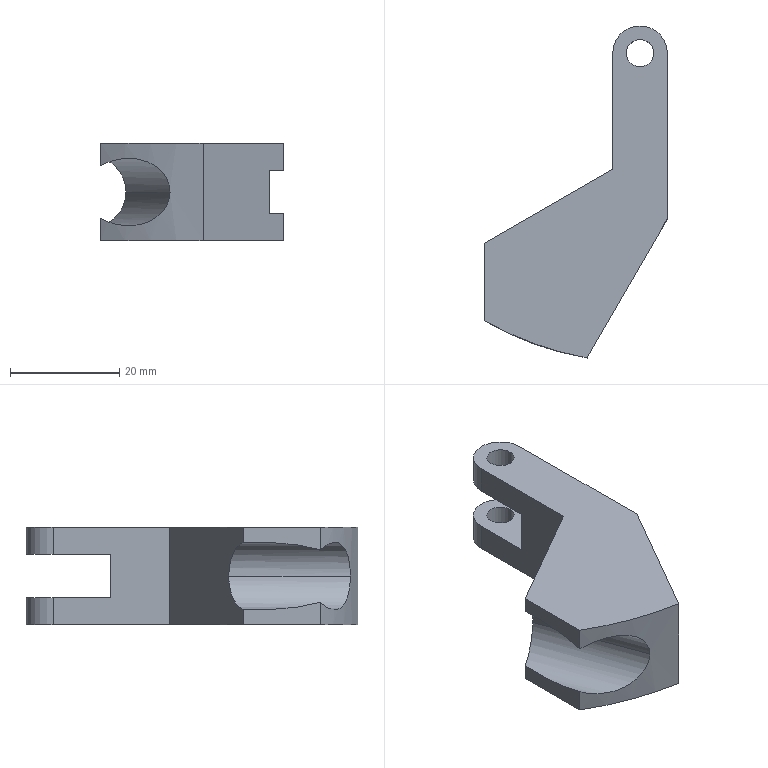Part | SolidWorks | features ICE 3, Extrusion 1 | 1 solid | 22 faces | box 33.5 x 60.913 x 17.9 mm | volume 14389 mm3 | plane 13 | cylinder 9 | commonest cylinder face diameters 5 x4 10 x2 12.4 x2 113.5 x1
STEP:
#1=CARTESIAN_POINT('',(-23.888,-32.221,8.95));
#2=VERTEX_POINT('',#1);
#3=CARTESIAN_POINT('',(-28.5,-34.884,15.076));
#4=VERTEX_POINT('',#3);
#5=CARTESIAN_POINT('',(-23.888,-32.221,8.95));
#6=CARTESIAN_POINT('',(-23.888,-32.221,12.151));
#7=CARTESIAN_POINT('',(-25.719,-33.278,14.583));
#8=CARTESIAN_POINT('',(-28.5,-34.884,15.076));
#9=(BOUNDED_CURVE()B_SPLINE_CURVE(3,(#5,#6,#7,#8),.UNSPECIFIED.,.F.,.F.)B_SPLINE_CURVE_WITH_KNOTS((4,4),(3.142,4.558),.UNSPECIFIED.)CURVE()GEOMETRIC_REPRESENTATION_ITEM()RATIONAL_B_SPLINE_CURVE((1.,0.8398,0.8398,1.))REPRESENTATION_ITEM(''));
#10=EDGE_CURVE('',#2,#4,#9,.T.);
#11=ORIENTED_EDGE('',*,*,#10,.F.);
#12=CARTESIAN_POINT('',(-15.774,-54.514,8.95));
#13=VERTEX_POINT('',#12);
#14=CARTESIAN_POINT('',(-26.37,-25.401,8.95));
#15=DIRECTION('',(0.342,-0.9397,0.));
#16=VECTOR('',#15,1000.);
#17=LINE('',#14,#16);
#18=EDGE_CURVE('',#2,#13,#17,.T.);
#19=ORIENTED_EDGE('',*,*,#18,.T.);
#20=CARTESIAN_POINT('',(-28.5,-49.075,13.771));
#21=VERTEX_POINT('',#20);
#22=CARTESIAN_POINT('',(-28.5,-49.075,13.771));
#23=CARTESIAN_POINT('',(-27.942,-49.399,14.106));
#24=CARTESIAN_POINT('',(-27.36,-49.724,14.372));
#25=CARTESIAN_POINT('',(-26.454,-50.208,14.688));
#26=CARTESIAN_POINT('',(-26.146,-50.369,14.778));
#27=CARTESIAN_POINT('',(-25.52,-50.689,14.932));
#28=CARTESIAN_POINT('',(-25.2,-50.849,14.994));
#29=CARTESIAN_POINT('',(-24.233,-51.321,15.136));
#30=CARTESIAN_POINT('',(-23.583,-51.623,15.17));
#31=CARTESIAN_POINT('',(-22.602,-52.056,15.124));
#32=CARTESIAN_POINT('',(-22.274,-52.197,15.092));
#33=CARTESIAN_POINT('',(-21.615,-52.473,14.994));
#34=CARTESIAN_POINT('',(-21.283,-52.609,14.926));
#35=CARTESIAN_POINT('',(-20.304,-52.998,14.667));
#36=CARTESIAN_POINT('',(-19.671,-53.236,14.422));
#37=CARTESIAN_POINT('',(-18.761,-53.56,13.92));
#38=CARTESIAN_POINT('',(-18.467,-53.662,13.73));
#39=CARTESIAN_POINT('',(-17.911,-53.85,13.31));
#40=CARTESIAN_POINT('',(-17.648,-53.937,13.079));
#41=CARTESIAN_POINT('',(-17.157,-54.095,12.571));
#42=CARTESIAN_POINT('',(-16.929,-54.166,12.292));
#43=CARTESIAN_POINT('',(-16.531,-54.289,11.702));
#44=CARTESIAN_POINT('',(-16.358,-54.342,11.39));
#45=CARTESIAN_POINT('',(-16.071,-54.427,10.725));
#46=CARTESIAN_POINT('',(-15.96,-54.459,10.38));
#47=CARTESIAN_POINT('',(-15.85,-54.492,9.853));
#48=CARTESIAN_POINT('',(-15.822,-54.5,9.675));
#49=CARTESIAN_POINT('',(-15.784,-54.511,9.315));
#50=CARTESIAN_POINT('',(-15.774,-54.514,9.132));
#51=CARTESIAN_POINT('',(-15.774,-54.514,8.95));
#52=B_SPLINE_CURVE_WITH_KNOTS('',3,(#22,#23,#24,#25,#26,#27,#28,#29,#30,#31,#32,#33,#34,#35,#36,#37,#38,#39,#40,#41,#42,#43,#44,#45,#46,#47,#48,#49,#50,#51),.UNSPECIFIED.,.F.,.F.,(4,2,2,2,2,2,2,2,2,2,2,2,2,2,4),(0.,0.002149,0.003224,0.004298,0.006447,0.007522,0.008597,0.01075,0.01182,0.01289,0.01397,0.01504,0.01612,0.01666,0.01719),.UNSPECIFIED.);
#53=EDGE_CURVE('',#21,#13,#52,.T.);
#54=ORIENTED_EDGE('',*,*,#53,.F.);
#55=CARTESIAN_POINT('',(-28.5,-34.884,15.076));
#56=CARTESIAN_POINT('',(-28.5,-40.017,15.35));
#57=CARTESIAN_POINT('',(-28.5,-45.034,14.889));
#58=CARTESIAN_POINT('',(-28.5,-49.075,13.771));
#59=(BOUNDED_CURVE()B_SPLINE_CURVE(3,(#55,#56,#57,#58),.UNSPECIFIED.,.F.,.F.)B_SPLINE_CURVE_WITH_KNOTS((4,4),(4.558,5.392),.UNSPECIFIED.)CURVE()GEOMETRIC_REPRESENTATION_ITEM()RATIONAL_B_SPLINE_CURVE((1.,0.9428,0.9428,1.))REPRESENTATION_ITEM(''));
#60=EDGE_CURVE('',#4,#21,#59,.T.);
#61=ORIENTED_EDGE('',*,*,#60,.F.);
#62=EDGE_LOOP('',(#11,#19,#54,#61));
#63=FACE_OUTER_BOUND('',#62,.T.);
#64=CARTESIAN_POINT('',(-32.196,-27.522,8.95));
#65=DIRECTION('',(0.342,-0.9397,0.));
#66=DIRECTION('',(0.9397,0.342,0.));
#67=AXIS2_PLACEMENT_3D('',#64,#65,#66);
#68=CYLINDRICAL_SURFACE('',#67,6.2);
#69=ADVANCED_FACE('',(#63),#68,.F.);
#70=CARTESIAN_POINT('',(-2.5,0.,17.9));
#71=VERTEX_POINT('',#70);
#72=CARTESIAN_POINT('',(2.5,0.,17.9));
#73=VERTEX_POINT('',#72);
#74=CARTESIAN_POINT('',(0.,0.,17.9));
#75=DIRECTION('',(0.,0.,1.));
#76=DIRECTION('',(1.,0.,0.));
#77=AXIS2_PLACEMENT_3D('',#74,#75,#76);
#78=CIRCLE('',#77,2.5);
#79=EDGE_CURVE('',#71,#73,#78,.T.);
#80=ORIENTED_EDGE('',*,*,#79,.T.);
#81=CARTESIAN_POINT('',(2.5,0.,12.9));
#82=VERTEX_POINT('',#81);
#83=CARTESIAN_POINT('',(2.5,0.,17.9));
#84=DIRECTION('',(0.,0.,-1.));
#85=VECTOR('',#84,1000.);
#86=LINE('',#83,#85);
#87=EDGE_CURVE('',#73,#82,#86,.T.);
#88=ORIENTED_EDGE('',*,*,#87,.T.);
#89=CARTESIAN_POINT('',(-2.5,0.,12.9));
#90=VERTEX_POINT('',#89);
#91=CARTESIAN_POINT('',(0.,0.,12.9));
#92=DIRECTION('',(0.,0.,1.));
#93=DIRECTION('',(1.,0.,0.));
#94=AXIS2_PLACEMENT_3D('',#91,#92,#93);
#95=CIRCLE('',#94,2.5);
#96=EDGE_CURVE('',#90,#82,#95,.T.);
#97=ORIENTED_EDGE('',*,*,#96,.F.);
#98=CARTESIAN_POINT('',(-2.5,0.,17.9));
#99=DIRECTION('',(0.,0.,-1.));
#100=VECTOR('',#99,1000.);
#101=LINE('',#98,#100);
#102=EDGE_CURVE('',#71,#90,#101,.T.);
#103=ORIENTED_EDGE('',*,*,#102,.F.);
#104=EDGE_LOOP('',(#80,#88,#97,#103));
#105=FACE_OUTER_BOUND('',#104,.T.);
#106=CARTESIAN_POINT('',(0.,0.,17.9));
#107=DIRECTION('',(0.,0.,-1.));
#108=DIRECTION('',(-1.,0.,0.));
#109=AXIS2_PLACEMENT_3D('',#106,#107,#108);
#110=CYLINDRICAL_SURFACE('',#109,2.5);
#111=ADVANCED_FACE('',(#105),#110,.F.);
#112=CARTESIAN_POINT('',(2.5,0.,5.));
#113=VERTEX_POINT('',#112);
#114=CARTESIAN_POINT('',(-2.5,0.,5.));
#115=VERTEX_POINT('',#114);
#116=CARTESIAN_POINT('',(0.,0.,5.));
#117=DIRECTION('',(0.,0.,-1.));
#118=DIRECTION('',(-1.,0.,0.));
#119=AXIS2_PLACEMENT_3D('',#116,#117,#118);
#120=CIRCLE('',#119,2.5);
#121=EDGE_CURVE('',#113,#115,#120,.T.);
#122=ORIENTED_EDGE('',*,*,#121,.F.);
#123=CARTESIAN_POINT('',(2.5,0.,0.));
#124=VERTEX_POINT('',#123);
#125=CARTESIAN_POINT('',(2.5,0.,17.9));
#126=DIRECTION('',(0.,0.,-1.));
#127=VECTOR('',#126,1000.);
#128=LINE('',#125,#127);
#129=EDGE_CURVE('',#113,#124,#128,.T.);
#130=ORIENTED_EDGE('',*,*,#129,.T.);
#131=CARTESIAN_POINT('',(-2.5,0.,0.));
#132=VERTEX_POINT('',#131);
#133=CARTESIAN_POINT('',(0.,0.,0.));
#134=DIRECTION('',(0.,0.,1.));
#135=DIRECTION('',(1.,0.,0.));
#136=AXIS2_PLACEMENT_3D('',#133,#134,#135);
#137=CIRCLE('',#136,2.5);
#138=EDGE_CURVE('',#132,#124,#137,.T.);
#139=ORIENTED_EDGE('',*,*,#138,.F.);
#140=CARTESIAN_POINT('',(-2.5,0.,17.9));
#141=DIRECTION('',(0.,0.,-1.));
#142=VECTOR('',#141,1000.);
#143=LINE('',#140,#142);
#144=EDGE_CURVE('',#115,#132,#143,.T.);
#145=ORIENTED_EDGE('',*,*,#144,.F.);
#146=EDGE_LOOP('',(#122,#130,#139,#145));
#147=FACE_OUTER_BOUND('',#146,.T.);
#148=CARTESIAN_POINT('',(0.,0.,17.9));
#149=DIRECTION('',(0.,0.,-1.));
#150=DIRECTION('',(-1.,0.,0.));
#151=AXIS2_PLACEMENT_3D('',#148,#149,#150);
#152=CYLINDRICAL_SURFACE('',#151,2.5);
#153=ADVANCED_FACE('',(#147),#152,.F.);
#154=CARTESIAN_POINT('',(-28.5,-49.075,4.129));
#155=VERTEX_POINT('',#154);
#156=CARTESIAN_POINT('',(-28.5,-49.075,0.));
#157=VERTEX_POINT('',#156);
#158=CARTESIAN_POINT('',(-28.5,-49.075,17.9));
#159=DIRECTION('',(0.,0.,-1.));
#160=VECTOR('',#159,1000.);
#161=LINE('',#158,#160);
#162=EDGE_CURVE('',#155,#157,#161,.T.);
#163=ORIENTED_EDGE('',*,*,#162,.F.);
#164=CARTESIAN_POINT('',(-28.5,-34.884,2.824));
#165=VERTEX_POINT('',#164);
#166=CARTESIAN_POINT('',(-28.5,-49.075,4.129));
#167=CARTESIAN_POINT('',(-28.5,-45.034,3.011));
#168=CARTESIAN_POINT('',(-28.5,-40.017,2.55));
#169=CARTESIAN_POINT('',(-28.5,-34.884,2.824));
#170=(BOUNDED_CURVE()B_SPLINE_CURVE(3,(#166,#167,#168,#169),.UNSPECIFIED.,.F.,.T.)B_SPLINE_CURVE_WITH_KNOTS((4,4),(0.8909,1.726),.UNSPECIFIED.)CURVE()GEOMETRIC_REPRESENTATION_ITEM()RATIONAL_B_SPLINE_CURVE((1.,0.9428,0.9428,1.))REPRESENTATION_ITEM(''));
#171=EDGE_CURVE('',#155,#165,#170,.T.);
#172=ORIENTED_EDGE('',*,*,#171,.T.);
#173=CARTESIAN_POINT('',(-28.5,-34.884,0.));
#174=VERTEX_POINT('',#173);
#175=CARTESIAN_POINT('',(-28.5,-34.884,17.9));
#176=DIRECTION('',(0.,0.,-1.));
#177=VECTOR('',#176,1000.);
#178=LINE('',#175,#177);
#179=EDGE_CURVE('',#165,#174,#178,.T.);
#180=ORIENTED_EDGE('',*,*,#179,.T.);
#181=CARTESIAN_POINT('',(-28.5,-34.884,0.));
#182=DIRECTION('',(0.,-1.,0.));
#183=VECTOR('',#182,1000.);
#184=LINE('',#181,#183);
#185=EDGE_CURVE('',#174,#157,#184,.T.);
#186=ORIENTED_EDGE('',*,*,#185,.T.);
#187=EDGE_LOOP('',(#163,#172,#180,#186));
#188=FACE_OUTER_BOUND('',#187,.T.);
#189=CARTESIAN_POINT('',(-28.5,-34.884,17.9));
#190=DIRECTION('',(1.,0.,0.));
#191=DIRECTION('',(0.,0.,-1.));
#192=AXIS2_PLACEMENT_3D('',#189,#190,#191);
#193=PLANE('',#192);
#194=ADVANCED_FACE('',(#188),#193,.F.);
#195=CARTESIAN_POINT('',(5.,0.,5.));
#196=VERTEX_POINT('',#195);
#197=CARTESIAN_POINT('',(5.,0.,0.));
#198=VERTEX_POINT('',#197);
#199=CARTESIAN_POINT('',(5.,0.,17.9));
#200=DIRECTION('',(0.,0.,-1.));
#201=VECTOR('',#200,1000.);
#202=LINE('',#199,#201);
#203=EDGE_CURVE('',#196,#198,#202,.T.);
#204=ORIENTED_EDGE('',*,*,#203,.F.);
#205=CARTESIAN_POINT('',(5.,-30.431,5.));
#206=VERTEX_POINT('',#205);
#207=CARTESIAN_POINT('',(5.,-30.431,5.));
#208=DIRECTION('',(0.,-1.,0.));
#209=VECTOR('',#208,1000.);
#210=LINE('',#207,#209);
#211=EDGE_CURVE('',#196,#206,#210,.T.);
#212=ORIENTED_EDGE('',*,*,#211,.T.);
#213=CARTESIAN_POINT('',(5.,-30.431,0.));
#214=VERTEX_POINT('',#213);
#215=CARTESIAN_POINT('',(5.,-30.431,17.9));
#216=DIRECTION('',(0.,0.,-1.));
#217=VECTOR('',#216,1000.);
#218=LINE('',#215,#217);
#219=EDGE_CURVE('',#206,#214,#218,.T.);
#220=ORIENTED_EDGE('',*,*,#219,.T.);
#221=CARTESIAN_POINT('',(5.,-30.431,0.));
#222=DIRECTION('',(0.,1.,0.));
#223=VECTOR('',#222,1000.);
#224=LINE('',#221,#223);
#225=EDGE_CURVE('',#214,#198,#224,.T.);
#226=ORIENTED_EDGE('',*,*,#225,.T.);
#227=EDGE_LOOP('',(#204,#212,#220,#226));
#228=FACE_OUTER_BOUND('',#227,.T.);
#229=CARTESIAN_POINT('',(5.,-30.431,17.9));
#230=DIRECTION('',(-1.,0.,0.));
#231=DIRECTION('',(0.,-1.,0.));
#232=AXIS2_PLACEMENT_3D('',#229,#230,#231);
#233=PLANE('',#232);
#234=ADVANCED_FACE('',(#228),#233,.F.);
#235=CARTESIAN_POINT('',(-5.,0.,5.));
#236=VERTEX_POINT('',#235);
#237=CARTESIAN_POINT('',(-5.,0.,0.));
#238=VERTEX_POINT('',#237);
#239=CARTESIAN_POINT('',(-5.,0.,17.9));
#240=DIRECTION('',(0.,0.,-1.));
#241=VECTOR('',#240,1000.);
#242=LINE('',#239,#241);
#243=EDGE_CURVE('',#236,#238,#242,.T.);
#244=ORIENTED_EDGE('',*,*,#243,.F.);
#245=CARTESIAN_POINT('',(0.,0.,5.));
#246=DIRECTION('',(0.,0.,-1.));
#247=DIRECTION('',(-1.,0.,0.));
#248=AXIS2_PLACEMENT_3D('',#245,#246,#247);
#249=CIRCLE('',#248,5.);
#250=EDGE_CURVE('',#236,#196,#249,.T.);
#251=ORIENTED_EDGE('',*,*,#250,.T.);
#252=ORIENTED_EDGE('',*,*,#203,.T.);
#253=CARTESIAN_POINT('',(0.,0.,0.));
#254=DIRECTION('',(0.,0.,1.));
#255=DIRECTION('',(1.,0.,0.));
#256=AXIS2_PLACEMENT_3D('',#253,#254,#255);
#257=CIRCLE('',#256,5.);
#258=EDGE_CURVE('',#198,#238,#257,.T.);
#259=ORIENTED_EDGE('',*,*,#258,.T.);
#260=EDGE_LOOP('',(#244,#251,#252,#259));
#261=FACE_OUTER_BOUND('',#260,.T.);
#262=CARTESIAN_POINT('',(0.,0.,17.9));
#263=DIRECTION('',(0.,0.,-1.));
#264=DIRECTION('',(-1.,0.,0.));
#265=AXIS2_PLACEMENT_3D('',#262,#263,#264);
#266=CYLINDRICAL_SURFACE('',#265,5.);
#267=ADVANCED_FACE('',(#261),#266,.T.);
#268=ORIENTED_EDGE('',*,*,#129,.F.);
#269=CARTESIAN_POINT('',(0.,0.,5.));
#270=DIRECTION('',(0.,0.,-1.));
#271=DIRECTION('',(-1.,0.,0.));
#272=AXIS2_PLACEMENT_3D('',#269,#270,#271);
#273=CIRCLE('',#272,2.5);
#274=EDGE_CURVE('',#115,#113,#273,.T.);
#275=ORIENTED_EDGE('',*,*,#274,.F.);
#276=ORIENTED_EDGE('',*,*,#144,.T.);
#277=CARTESIAN_POINT('',(0.,0.,0.));
#278=DIRECTION('',(0.,0.,1.));
#279=DIRECTION('',(1.,0.,0.));
#280=AXIS2_PLACEMENT_3D('',#277,#278,#279);
#281=CIRCLE('',#280,2.5);
#282=EDGE_CURVE('',#124,#132,#281,.T.);
#283=ORIENTED_EDGE('',*,*,#282,.F.);
#284=EDGE_LOOP('',(#268,#275,#276,#283));
#285=FACE_OUTER_BOUND('',#284,.T.);
#286=CARTESIAN_POINT('',(0.,0.,17.9));
#287=DIRECTION('',(0.,0.,-1.));
#288=DIRECTION('',(-1.,0.,0.));
#289=AXIS2_PLACEMENT_3D('',#286,#287,#288);
#290=CYLINDRICAL_SURFACE('',#289,2.5);
#291=ADVANCED_FACE('',(#285),#290,.F.);
#292=CARTESIAN_POINT('',(5.,-30.431,12.9));
#293=VERTEX_POINT('',#292);
#294=CARTESIAN_POINT('',(2.55,-34.675,12.9));
#295=VERTEX_POINT('',#294);
#296=CARTESIAN_POINT('',(2.55,-34.675,12.9));
#297=DIRECTION('',(-0.5,-0.866,0.));
#298=VECTOR('',#297,1000.);
#299=LINE('',#296,#298);
#300=EDGE_CURVE('',#293,#295,#299,.T.);
#301=ORIENTED_EDGE('',*,*,#300,.F.);
#302=CARTESIAN_POINT('',(5.,-30.431,17.9));
#303=VERTEX_POINT('',#302);
#304=CARTESIAN_POINT('',(5.,-30.431,17.9));
#305=DIRECTION('',(0.,0.,-1.));
#306=VECTOR('',#305,1000.);
#307=LINE('',#304,#306);
#308=EDGE_CURVE('',#303,#293,#307,.T.);
#309=ORIENTED_EDGE('',*,*,#308,.F.);
#310=CARTESIAN_POINT('',(-9.712,-55.913,17.9));
#311=VERTEX_POINT('',#310);
#312=CARTESIAN_POINT('',(-9.712,-55.913,17.9));
#313=DIRECTION('',(0.5,0.866,0.));
#314=VECTOR('',#313,1000.);
#315=LINE('',#312,#314);
#316=EDGE_CURVE('',#311,#303,#315,.T.);
#317=ORIENTED_EDGE('',*,*,#316,.F.);
#318=CARTESIAN_POINT('',(-9.712,-55.913,0.));
#319=VERTEX_POINT('',#318);
#320=CARTESIAN_POINT('',(-9.712,-55.913,17.9));
#321=DIRECTION('',(0.,0.,-1.));
#322=VECTOR('',#321,1000.);
#323=LINE('',#320,#322);
#324=EDGE_CURVE('',#311,#319,#323,.T.);
#325=ORIENTED_EDGE('',*,*,#324,.T.);
#326=CARTESIAN_POINT('',(-9.712,-55.913,0.));
#327=DIRECTION('',(0.5,0.866,0.));
#328=VECTOR('',#327,1000.);
#329=LINE('',#326,#328);
#330=EDGE_CURVE('',#319,#214,#329,.T.);
#331=ORIENTED_EDGE('',*,*,#330,.T.);
#332=ORIENTED_EDGE('',*,*,#219,.F.);
#333=CARTESIAN_POINT('',(2.55,-34.675,5.));
#334=VERTEX_POINT('',#333);
#335=CARTESIAN_POINT('',(2.55,-34.675,5.));
#336=DIRECTION('',(-0.5,-0.866,0.));
#337=VECTOR('',#336,1000.);
#338=LINE('',#335,#337);
#339=EDGE_CURVE('',#206,#334,#338,.T.);
#340=ORIENTED_EDGE('',*,*,#339,.T.);
#341=CARTESIAN_POINT('',(2.55,-34.675,12.9));
#342=DIRECTION('',(0.,0.,-1.));
#343=VECTOR('',#342,1000.);
#344=LINE('',#341,#343);
#345=EDGE_CURVE('',#295,#334,#344,.T.);
#346=ORIENTED_EDGE('',*,*,#345,.F.);
#347=EDGE_LOOP('',(#301,#309,#317,#325,#331,#332,#340,#346));
#348=FACE_OUTER_BOUND('',#347,.T.);
#349=CARTESIAN_POINT('',(-9.712,-55.913,17.9));
#350=DIRECTION('',(-0.866,0.5,0.));
#351=DIRECTION('',(-0.5,-0.866,0.));
#352=AXIS2_PLACEMENT_3D('',#349,#350,#351);
#353=PLANE('',#352);
#354=ADVANCED_FACE('',(#348),#353,.F.);
#355=CARTESIAN_POINT('',(5.,0.,12.9));
#356=VERTEX_POINT('',#355);
#357=CARTESIAN_POINT('',(5.,-30.431,12.9));
#358=DIRECTION('',(0.,-1.,0.));
#359=VECTOR('',#358,1000.);
#360=LINE('',#357,#359);
#361=EDGE_CURVE('',#356,#293,#360,.T.);
#362=ORIENTED_EDGE('',*,*,#361,.F.);
#363=CARTESIAN_POINT('',(5.,0.,17.9));
#364=VERTEX_POINT('',#363);
#365=CARTESIAN_POINT('',(5.,0.,17.9));
#366=DIRECTION('',(0.,0.,-1.));
#367=VECTOR('',#366,1000.);
#368=LINE('',#365,#367);
#369=EDGE_CURVE('',#364,#356,#368,.T.);
#370=ORIENTED_EDGE('',*,*,#369,.F.);
#371=CARTESIAN_POINT('',(5.,-30.431,17.9));
#372=DIRECTION('',(0.,1.,0.));
#373=VECTOR('',#372,1000.);
#374=LINE('',#371,#373);
#375=EDGE_CURVE('',#303,#364,#374,.T.);
#376=ORIENTED_EDGE('',*,*,#375,.F.);
#377=ORIENTED_EDGE('',*,*,#308,.T.);
#378=EDGE_LOOP('',(#362,#370,#376,#377));
#379=FACE_OUTER_BOUND('',#378,.T.);
#380=CARTESIAN_POINT('',(5.,-30.431,17.9));
#381=DIRECTION('',(-1.,0.,0.));
#382=DIRECTION('',(0.,-1.,0.));
#383=AXIS2_PLACEMENT_3D('',#380,#381,#382);
#384=PLANE('',#383);
#385=ADVANCED_FACE('',(#379),#384,.F.);
#386=CARTESIAN_POINT('',(-5.,0.,17.9));
#387=VERTEX_POINT('',#386);
#388=CARTESIAN_POINT('',(0.,0.,17.9));
#389=DIRECTION('',(0.,0.,1.));
#390=DIRECTION('',(1.,0.,0.));
#391=AXIS2_PLACEMENT_3D('',#388,#389,#390);
#392=CIRCLE('',#391,5.);
#393=EDGE_CURVE('',#364,#387,#392,.T.);
#394=ORIENTED_EDGE('',*,*,#393,.T.);
#395=CARTESIAN_POINT('',(-5.,-21.316,17.9));
#396=VERTEX_POINT('',#395);
#397=CARTESIAN_POINT('',(-5.,0.,17.9));
#398=DIRECTION('',(0.,-1.,0.));
#399=VECTOR('',#398,1000.);
#400=LINE('',#397,#399);
#401=EDGE_CURVE('',#387,#396,#400,.T.);
#402=ORIENTED_EDGE('',*,*,#401,.T.);
#403=CARTESIAN_POINT('',(-28.5,-34.884,17.9));
#404=VERTEX_POINT('',#403);
#405=CARTESIAN_POINT('',(-5.,-21.316,17.9));
#406=DIRECTION('',(-0.866,-0.5,0.));
#407=VECTOR('',#406,1000.);
#408=LINE('',#405,#407);
#409=EDGE_CURVE('',#396,#404,#408,.T.);
#410=ORIENTED_EDGE('',*,*,#409,.T.);
#411=CARTESIAN_POINT('',(-28.5,-49.075,17.9));
#412=VERTEX_POINT('',#411);
#413=CARTESIAN_POINT('',(-28.5,-34.884,17.9));
#414=DIRECTION('',(0.,-1.,0.));
#415=VECTOR('',#414,1000.);
#416=LINE('',#413,#415);
#417=EDGE_CURVE('',#404,#412,#416,.T.);
#418=ORIENTED_EDGE('',*,*,#417,.T.);
#419=CARTESIAN_POINT('',(0.,0.,17.9));
#420=DIRECTION('',(0.,0.,1.));
#421=DIRECTION('',(1.,0.,0.));
#422=AXIS2_PLACEMENT_3D('',#419,#420,#421);
#423=CIRCLE('',#422,56.75);
#424=EDGE_CURVE('',#412,#311,#423,.T.);
#425=ORIENTED_EDGE('',*,*,#424,.T.);
#426=ORIENTED_EDGE('',*,*,#316,.T.);
#427=ORIENTED_EDGE('',*,*,#375,.T.);
#428=EDGE_LOOP('',(#394,#402,#410,#418,#425,#426,#427));
#429=FACE_OUTER_BOUND('',#428,.T.);
#430=ORIENTED_EDGE('',*,*,#79,.F.);
#431=CARTESIAN_POINT('',(0.,0.,17.9));
#432=DIRECTION('',(0.,0.,1.));
#433=DIRECTION('',(1.,0.,0.));
#434=AXIS2_PLACEMENT_3D('',#431,#432,#433);
#435=CIRCLE('',#434,2.5);
#436=EDGE_CURVE('',#73,#71,#435,.T.);
#437=ORIENTED_EDGE('',*,*,#436,.F.);
#438=EDGE_LOOP('',(#430,#437));
#439=FACE_BOUND('',#438,.T.);
#440=CARTESIAN_POINT('',(0.,0.,17.9));
#441=DIRECTION('',(0.,0.,1.));
#442=DIRECTION('',(1.,0.,0.));
#443=AXIS2_PLACEMENT_3D('',#440,#441,#442);
#444=PLANE('',#443);
#445=ADVANCED_FACE('',(#429,#439),#444,.T.);
#446=ORIENTED_EDGE('',*,*,#258,.F.);
#447=ORIENTED_EDGE('',*,*,#225,.F.);
#448=ORIENTED_EDGE('',*,*,#330,.F.);
#449=CARTESIAN_POINT('',(0.,0.,0.));
#450=DIRECTION('',(0.,0.,1.));
#451=DIRECTION('',(1.,0.,0.));
#452=AXIS2_PLACEMENT_3D('',#449,#450,#451);
#453=CIRCLE('',#452,56.75);
#454=EDGE_CURVE('',#157,#319,#453,.T.);
#455=ORIENTED_EDGE('',*,*,#454,.F.);
#456=ORIENTED_EDGE('',*,*,#185,.F.);
#457=CARTESIAN_POINT('',(-5.,-21.316,0.));
#458=VERTEX_POINT('',#457);
#459=CARTESIAN_POINT('',(-5.,-21.316,0.));
#460=DIRECTION('',(-0.866,-0.5,0.));
#461=VECTOR('',#460,1000.);
#462=LINE('',#459,#461);
#463=EDGE_CURVE('',#458,#174,#462,.T.);
#464=ORIENTED_EDGE('',*,*,#463,.F.);
#465=CARTESIAN_POINT('',(-5.,0.,0.));
#466=DIRECTION('',(0.,-1.,0.));
#467=VECTOR('',#466,1000.);
#468=LINE('',#465,#467);
#469=EDGE_CURVE('',#238,#458,#468,.T.);
#470=ORIENTED_EDGE('',*,*,#469,.F.);
#471=EDGE_LOOP('',(#446,#447,#448,#455,#456,#464,#470));
#472=FACE_OUTER_BOUND('',#471,.T.);
#473=ORIENTED_EDGE('',*,*,#138,.T.);
#474=ORIENTED_EDGE('',*,*,#282,.T.);
#475=EDGE_LOOP('',(#473,#474));
#476=FACE_BOUND('',#475,.T.);
#477=CARTESIAN_POINT('',(0.,0.,0.));
#478=DIRECTION('',(0.,0.,1.));
#479=DIRECTION('',(1.,0.,0.));
#480=AXIS2_PLACEMENT_3D('',#477,#478,#479);
#481=PLANE('',#480);
#482=ADVANCED_FACE('',(#472,#476),#481,.F.);
#483=ORIENTED_EDGE('',*,*,#369,.T.);
#484=CARTESIAN_POINT('',(-5.,0.,12.9));
#485=VERTEX_POINT('',#484);
#486=CARTESIAN_POINT('',(0.,0.,12.9));
#487=DIRECTION('',(0.,0.,1.));
#488=DIRECTION('',(1.,0.,0.));
#489=AXIS2_PLACEMENT_3D('',#486,#487,#488);
#490=CIRCLE('',#489,5.);
#491=EDGE_CURVE('',#356,#485,#490,.T.);
#492=ORIENTED_EDGE('',*,*,#491,.T.);
#493=CARTESIAN_POINT('',(-5.,0.,17.9));
#494=DIRECTION('',(0.,0.,-1.));
#495=VECTOR('',#494,1000.);
#496=LINE('',#493,#495);
#497=EDGE_CURVE('',#387,#485,#496,.T.);
#498=ORIENTED_EDGE('',*,*,#497,.F.);
#499=ORIENTED_EDGE('',*,*,#393,.F.);
#500=EDGE_LOOP('',(#483,#492,#498,#499));
#501=FACE_OUTER_BOUND('',#500,.T.);
#502=CARTESIAN_POINT('',(0.,0.,17.9));
#503=DIRECTION('',(0.,0.,-1.));
#504=DIRECTION('',(-1.,0.,0.));
#505=AXIS2_PLACEMENT_3D('',#502,#503,#504);
#506=CYLINDRICAL_SURFACE('',#505,5.);
#507=ADVANCED_FACE('',(#501),#506,.T.);
#508=CARTESIAN_POINT('',(-5.,-10.556,5.));
#509=VERTEX_POINT('',#508);
#510=CARTESIAN_POINT('',(-5.,-10.556,12.9));
#511=VERTEX_POINT('',#510);
#512=CARTESIAN_POINT('',(-5.,-10.556,5.));
#513=DIRECTION('',(0.,0.,1.));
#514=VECTOR('',#513,1000.);
#515=LINE('',#512,#514);
#516=EDGE_CURVE('',#509,#511,#515,.T.);
#517=ORIENTED_EDGE('',*,*,#516,.F.);
#518=CARTESIAN_POINT('',(-5.,-10.556,5.));
#519=DIRECTION('',(0.,-1.,0.));
#520=VECTOR('',#519,1000.);
#521=LINE('',#518,#520);
#522=EDGE_CURVE('',#236,#509,#521,.T.);
#523=ORIENTED_EDGE('',*,*,#522,.F.);
#524=ORIENTED_EDGE('',*,*,#243,.T.);
#525=ORIENTED_EDGE('',*,*,#469,.T.);
#526=CARTESIAN_POINT('',(-5.,-21.316,17.9));
#527=DIRECTION('',(0.,0.,-1.));
#528=VECTOR('',#527,1000.);
#529=LINE('',#526,#528);
#530=EDGE_CURVE('',#396,#458,#529,.T.);
#531=ORIENTED_EDGE('',*,*,#530,.F.);
#532=ORIENTED_EDGE('',*,*,#401,.F.);
#533=ORIENTED_EDGE('',*,*,#497,.T.);
#534=CARTESIAN_POINT('',(-5.,7.33,12.9));
#535=DIRECTION('',(0.,1.,0.));
#536=VECTOR('',#535,1000.);
#537=LINE('',#534,#536);
#538=EDGE_CURVE('',#511,#485,#537,.T.);
#539=ORIENTED_EDGE('',*,*,#538,.F.);
#540=EDGE_LOOP('',(#517,#523,#524,#525,#531,#532,#533,#539));
#541=FACE_OUTER_BOUND('',#540,.T.);
#542=CARTESIAN_POINT('',(-5.,0.,17.9));
#543=DIRECTION('',(1.,0.,0.));
#544=DIRECTION('',(0.,1.,0.));
#545=AXIS2_PLACEMENT_3D('',#542,#543,#544);
#546=PLANE('',#545);
#547=ADVANCED_FACE('',(#541),#546,.F.);
#548=ORIENTED_EDGE('',*,*,#179,.F.);
#549=CARTESIAN_POINT('',(-28.5,-34.884,2.824));
#550=CARTESIAN_POINT('',(-25.719,-33.278,3.317));
#551=CARTESIAN_POINT('',(-23.888,-32.221,5.749));
#552=CARTESIAN_POINT('',(-23.888,-32.221,8.95));
#553=(BOUNDED_CURVE()B_SPLINE_CURVE(3,(#549,#550,#551,#552),.UNSPECIFIED.,.F.,.F.)B_SPLINE_CURVE_WITH_KNOTS((4,4),(1.726,3.142),.UNSPECIFIED.)CURVE()GEOMETRIC_REPRESENTATION_ITEM()RATIONAL_B_SPLINE_CURVE((1.,0.8398,0.8398,1.))REPRESENTATION_ITEM(''));
#554=EDGE_CURVE('',#165,#2,#553,.T.);
#555=ORIENTED_EDGE('',*,*,#554,.T.);
#556=ORIENTED_EDGE('',*,*,#10,.T.);
#557=CARTESIAN_POINT('',(-28.5,-34.884,17.9));
#558=DIRECTION('',(0.,0.,-1.));
#559=VECTOR('',#558,1000.);
#560=LINE('',#557,#559);
#561=EDGE_CURVE('',#404,#4,#560,.T.);
#562=ORIENTED_EDGE('',*,*,#561,.F.);
#563=ORIENTED_EDGE('',*,*,#409,.F.);
#564=ORIENTED_EDGE('',*,*,#530,.T.);
#565=ORIENTED_EDGE('',*,*,#463,.T.);
#566=EDGE_LOOP('',(#548,#555,#556,#562,#563,#564,#565));
#567=FACE_OUTER_BOUND('',#566,.T.);
#568=CARTESIAN_POINT('',(-5.,-21.316,17.9));
#569=DIRECTION('',(0.5,-0.866,0.));
#570=DIRECTION('',(0.866,0.5,0.));
#571=AXIS2_PLACEMENT_3D('',#568,#569,#570);
#572=PLANE('',#571);
#573=ADVANCED_FACE('',(#567),#572,.F.);
#574=ORIENTED_EDGE('',*,*,#561,.T.);
#575=ORIENTED_EDGE('',*,*,#60,.T.);
#576=CARTESIAN_POINT('',(-28.5,-49.075,17.9));
#577=DIRECTION('',(0.,0.,-1.));
#578=VECTOR('',#577,1000.);
#579=LINE('',#576,#578);
#580=EDGE_CURVE('',#412,#21,#579,.T.);
#581=ORIENTED_EDGE('',*,*,#580,.F.);
#582=ORIENTED_EDGE('',*,*,#417,.F.);
#583=EDGE_LOOP('',(#574,#575,#581,#582));
#584=FACE_OUTER_BOUND('',#583,.T.);
#585=CARTESIAN_POINT('',(-28.5,-34.884,17.9));
#586=DIRECTION('',(1.,0.,0.));
#587=DIRECTION('',(0.,0.,-1.));
#588=AXIS2_PLACEMENT_3D('',#585,#586,#587);
#589=PLANE('',#588);
#590=ADVANCED_FACE('',(#584),#589,.F.);
#591=ORIENTED_EDGE('',*,*,#580,.T.);
#592=ORIENTED_EDGE('',*,*,#53,.T.);
#593=CARTESIAN_POINT('',(-15.774,-54.514,8.95));
#594=CARTESIAN_POINT('',(-15.774,-54.514,8.586));
#595=CARTESIAN_POINT('',(-15.812,-54.503,8.228));
#596=CARTESIAN_POINT('',(-15.96,-54.46,7.523));
#597=CARTESIAN_POINT('',(-16.071,-54.427,7.174));
#598=CARTESIAN_POINT('',(-16.355,-54.342,6.516));
#599=CARTESIAN_POINT('',(-16.527,-54.29,6.203));
#600=CARTESIAN_POINT('',(-16.929,-54.166,5.608));
#601=CARTESIAN_POINT('',(-17.154,-54.096,5.333));
#602=CARTESIAN_POINT('',(-17.643,-53.938,4.826));
#603=CARTESIAN_POINT('',(-17.909,-53.851,4.591));
#604=CARTESIAN_POINT('',(-18.467,-53.662,4.17));
#605=CARTESIAN_POINT('',(-18.758,-53.561,3.983));
#606=CARTESIAN_POINT('',(-19.357,-53.348,3.651));
#607=CARTESIAN_POINT('',(-19.666,-53.235,3.506));
#608=CARTESIAN_POINT('',(-20.302,-52.995,3.254));
#609=CARTESIAN_POINT('',(-20.626,-52.87,3.148));
#610=CARTESIAN_POINT('',(-21.599,-52.484,2.89));
#611=CARTESIAN_POINT('',(-22.254,-52.21,2.793));
#612=CARTESIAN_POINT('',(-23.243,-51.773,2.746));
#613=CARTESIAN_POINT('',(-23.574,-51.623,2.746));
#614=CARTESIAN_POINT('',(-24.227,-51.32,2.779));
#615=CARTESIAN_POINT('',(-24.55,-51.166,2.811));
#616=CARTESIAN_POINT('',(-25.19,-50.854,2.904));
#617=CARTESIAN_POINT('',(-25.506,-50.696,2.965));
#618=CARTESIAN_POINT('',(-26.133,-50.376,3.118));
#619=CARTESIAN_POINT('',(-26.445,-50.213,3.209));
#620=CARTESIAN_POINT('',(-27.359,-49.725,3.527));
#621=CARTESIAN_POINT('',(-27.943,-49.398,3.795));
#622=CARTESIAN_POINT('',(-28.5,-49.075,4.129));
#623=B_SPLINE_CURVE_WITH_KNOTS('',3,(#593,#594,#595,#596,#597,#598,#599,#600,#601,#602,#603,#604,#605,#606,#607,#608,#609,#610,#611,#612,#613,#614,#615,#616,#617,#618,#619,#620,#621,#622),.UNSPECIFIED.,.F.,.F.,(4,2,2,2,2,2,2,2,2,2,2,2,2,2,4),(0.01719,0.01826,0.01934,0.02041,0.02148,0.02255,0.02362,0.0247,0.02577,0.02791,0.02898,0.03005,0.03113,0.0322,0.03434),.UNSPECIFIED.);
#624=EDGE_CURVE('',#13,#155,#623,.T.);
#625=ORIENTED_EDGE('',*,*,#624,.T.);
#626=ORIENTED_EDGE('',*,*,#162,.T.);
#627=ORIENTED_EDGE('',*,*,#454,.T.);
#628=ORIENTED_EDGE('',*,*,#324,.F.);
#629=ORIENTED_EDGE('',*,*,#424,.F.);
#630=EDGE_LOOP('',(#591,#592,#625,#626,#627,#628,#629));
#631=FACE_OUTER_BOUND('',#630,.T.);
#632=CARTESIAN_POINT('',(0.,0.,17.9));
#633=DIRECTION('',(0.,0.,-1.));
#634=DIRECTION('',(-1.,0.,0.));
#635=AXIS2_PLACEMENT_3D('',#632,#633,#634);
#636=CYLINDRICAL_SURFACE('',#635,56.75);
#637=ADVANCED_FACE('',(#631),#636,.T.);
#638=ORIENTED_EDGE('',*,*,#87,.F.);
#639=ORIENTED_EDGE('',*,*,#436,.T.);
#640=ORIENTED_EDGE('',*,*,#102,.T.);
#641=CARTESIAN_POINT('',(0.,0.,12.9));
#642=DIRECTION('',(0.,0.,1.));
#643=DIRECTION('',(1.,0.,0.));
#644=AXIS2_PLACEMENT_3D('',#641,#642,#643);
#645=CIRCLE('',#644,2.5);
#646=EDGE_CURVE('',#82,#90,#645,.T.);
#647=ORIENTED_EDGE('',*,*,#646,.F.);
#648=EDGE_LOOP('',(#638,#639,#640,#647));
#649=FACE_OUTER_BOUND('',#648,.T.);
#650=CARTESIAN_POINT('',(0.,0.,17.9));
#651=DIRECTION('',(0.,0.,-1.));
#652=DIRECTION('',(-1.,0.,0.));
#653=AXIS2_PLACEMENT_3D('',#650,#651,#652);
#654=CYLINDRICAL_SURFACE('',#653,2.5);
#655=ADVANCED_FACE('',(#649),#654,.F.);
#656=CARTESIAN_POINT('',(-1.703,-10.556,5.));
#657=VERTEX_POINT('',#656);
#658=CARTESIAN_POINT('',(-1.849,-9.729,5.));
#659=DIRECTION('',(-0.1736,0.9848,0.));
#660=VECTOR('',#659,1000.);
#661=LINE('',#658,#660);
#662=EDGE_CURVE('',#334,#657,#661,.T.);
#663=ORIENTED_EDGE('',*,*,#662,.T.);
#664=CARTESIAN_POINT('',(-1.703,-10.556,12.9));
#665=VERTEX_POINT('',#664);
#666=CARTESIAN_POINT('',(-1.703,-10.556,12.9));
#667=DIRECTION('',(0.,0.,1.));
#668=VECTOR('',#667,1000.);
#669=LINE('',#666,#668);
#670=EDGE_CURVE('',#657,#665,#669,.T.);
#671=ORIENTED_EDGE('',*,*,#670,.T.);
#672=CARTESIAN_POINT('',(-1.849,-9.729,12.9));
#673=DIRECTION('',(-0.1736,0.9848,0.));
#674=VECTOR('',#673,1000.);
#675=LINE('',#672,#674);
#676=EDGE_CURVE('',#295,#665,#675,.T.);
#677=ORIENTED_EDGE('',*,*,#676,.F.);
#678=ORIENTED_EDGE('',*,*,#345,.T.);
#679=EDGE_LOOP('',(#663,#671,#677,#678));
#680=FACE_OUTER_BOUND('',#679,.T.);
#681=CARTESIAN_POINT('',(-1.849,-9.729,12.9));
#682=DIRECTION('',(-0.9848,-0.1736,0.));
#683=DIRECTION('',(0.1736,-0.9848,0.));
#684=AXIS2_PLACEMENT_3D('',#681,#682,#683);
#685=PLANE('',#684);
#686=ADVANCED_FACE('',(#680),#685,.F.);
#687=ORIENTED_EDGE('',*,*,#491,.F.);
#688=ORIENTED_EDGE('',*,*,#361,.T.);
#689=ORIENTED_EDGE('',*,*,#300,.T.);
#690=ORIENTED_EDGE('',*,*,#676,.T.);
#691=CARTESIAN_POINT('',(36.9,-10.556,12.9));
#692=DIRECTION('',(-1.,0.,0.));
#693=VECTOR('',#692,1000.);
#694=LINE('',#691,#693);
#695=EDGE_CURVE('',#665,#511,#694,.T.);
#696=ORIENTED_EDGE('',*,*,#695,.T.);
#697=ORIENTED_EDGE('',*,*,#538,.T.);
#698=EDGE_LOOP('',(#687,#688,#689,#690,#696,#697));
#699=FACE_OUTER_BOUND('',#698,.T.);
#700=ORIENTED_EDGE('',*,*,#96,.T.);
#701=ORIENTED_EDGE('',*,*,#646,.T.);
#702=EDGE_LOOP('',(#700,#701));
#703=FACE_BOUND('',#702,.T.);
#704=CARTESIAN_POINT('',(0.,0.,12.9));
#705=DIRECTION('',(0.,0.,-1.));
#706=DIRECTION('',(-1.,0.,0.));
#707=AXIS2_PLACEMENT_3D('',#704,#705,#706);
#708=PLANE('',#707);
#709=ADVANCED_FACE('',(#699,#703),#708,.T.);
#710=ORIENTED_EDGE('',*,*,#211,.F.);
#711=ORIENTED_EDGE('',*,*,#250,.F.);
#712=ORIENTED_EDGE('',*,*,#522,.T.);
#713=CARTESIAN_POINT('',(36.9,-10.556,5.));
#714=DIRECTION('',(-1.,0.,0.));
#715=VECTOR('',#714,1000.);
#716=LINE('',#713,#715);
#717=EDGE_CURVE('',#657,#509,#716,.T.);
#718=ORIENTED_EDGE('',*,*,#717,.F.);
#719=ORIENTED_EDGE('',*,*,#662,.F.);
#720=ORIENTED_EDGE('',*,*,#339,.F.);
#721=EDGE_LOOP('',(#710,#711,#712,#718,#719,#720));
#722=FACE_OUTER_BOUND('',#721,.T.);
#723=ORIENTED_EDGE('',*,*,#274,.T.);
#724=ORIENTED_EDGE('',*,*,#121,.T.);
#725=EDGE_LOOP('',(#723,#724));
#726=FACE_BOUND('',#725,.T.);
#727=CARTESIAN_POINT('',(0.,0.,5.));
#728=DIRECTION('',(0.,0.,-1.));
#729=DIRECTION('',(-1.,0.,0.));
#730=AXIS2_PLACEMENT_3D('',#727,#728,#729);
#731=PLANE('',#730);
#732=ADVANCED_FACE('',(#722,#726),#731,.F.);
#733=ORIENTED_EDGE('',*,*,#717,.T.);
#734=ORIENTED_EDGE('',*,*,#516,.T.);
#735=ORIENTED_EDGE('',*,*,#695,.F.);
#736=ORIENTED_EDGE('',*,*,#670,.F.);
#737=EDGE_LOOP('',(#733,#734,#735,#736));
#738=FACE_OUTER_BOUND('',#737,.T.);
#739=CARTESIAN_POINT('',(36.9,-10.556,5.));
#740=DIRECTION('',(0.,-1.,0.));
#741=DIRECTION('',(1.,0.,0.));
#742=AXIS2_PLACEMENT_3D('',#739,#740,#741);
#743=PLANE('',#742);
#744=ADVANCED_FACE('',(#738),#743,.F.);
#745=ORIENTED_EDGE('',*,*,#18,.F.);
#746=ORIENTED_EDGE('',*,*,#554,.F.);
#747=ORIENTED_EDGE('',*,*,#171,.F.);
#748=ORIENTED_EDGE('',*,*,#624,.F.);
#749=EDGE_LOOP('',(#745,#746,#747,#748));
#750=FACE_OUTER_BOUND('',#749,.T.);
#751=CARTESIAN_POINT('',(-32.196,-27.522,8.95));
#752=DIRECTION('',(0.342,-0.9397,0.));
#753=DIRECTION('',(0.9397,0.342,0.));
#754=AXIS2_PLACEMENT_3D('',#751,#752,#753);
#755=CYLINDRICAL_SURFACE('',#754,6.2);
#756=ADVANCED_FACE('',(#750),#755,.F.);
#757=CLOSED_SHELL('',(#69,#111,#153,#194,#234,#267,#291,#354,#385,#445,#482,#507,#547,#573,#590,#637,#655,#686,#709,#732,#744,#756));
#758=MANIFOLD_SOLID_BREP('',#757);
#759=CARTESIAN_POINT('',(0.,0.,0.));
#760=DIRECTION('',(0.,0.,1.));
#761=DIRECTION('',(1.,0.,0.));
#762=AXIS2_PLACEMENT_3D('',#759,#760,#761);
#763=(LENGTH_UNIT()NAMED_UNIT(*)SI_UNIT(.MILLI.,.METRE.));
#764=UNCERTAINTY_MEASURE_WITH_UNIT(LENGTH_MEASURE(0.00001),#763,'','');
#765=(NAMED_UNIT(*)PLANE_ANGLE_UNIT()SI_UNIT($,.RADIAN.));
#766=(NAMED_UNIT(*)SI_UNIT($,.STERADIAN.)SOLID_ANGLE_UNIT());
#767=(GEOMETRIC_REPRESENTATION_CONTEXT(3)GLOBAL_UNCERTAINTY_ASSIGNED_CONTEXT((#764))GLOBAL_UNIT_ASSIGNED_CONTEXT((#763,#765,#766))REPRESENTATION_CONTEXT('',''));
#768=ADVANCED_BREP_SHAPE_REPRESENTATION('',(#758,#762),#767);